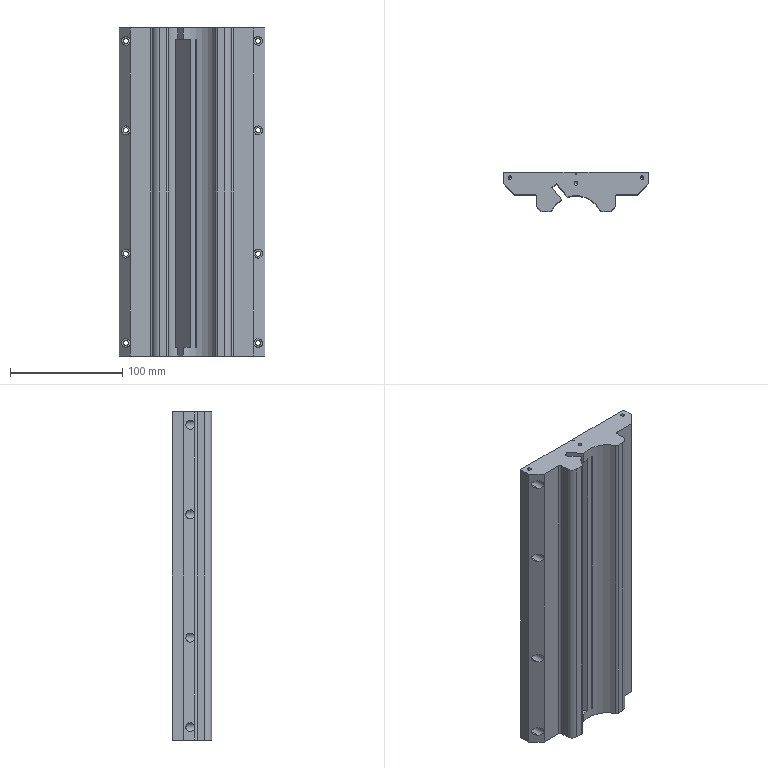Part | SolidWorks | features ICE 4, Fillet 3, HoleWzd 2, MirrorPattern 2, Chamfer 1, Cut 1, Extrusion 1, LPattern 1 | 1 solid | 96 faces | box 130 x 35 x 293 mm | volume 778685 mm3 | cylinder 52 | plane 40 | cone 4 | commonest cylinder face diameters 4.5 x16 8 x16 3.3 x12 4 x4 12 x2 48 x2